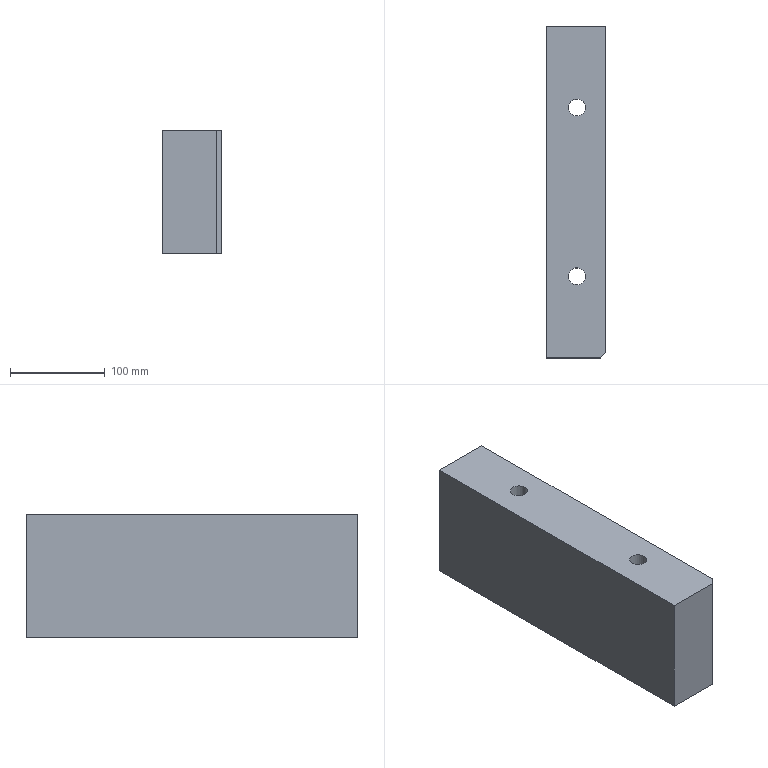Part | NX | features CC01 2 | 1 solid | 13 faces | box 63 x 350 x 130 mm | volume 2794571 mm3 | plane 7 | cylinder 4 | cone 2 | commonest cylinder face diameters 10 x2 18 x2
STEP:
#1=CARTESIAN_POINT('',(-137.5,142.,-240.5));
#2=VERTEX_POINT('',#1);
#3=CARTESIAN_POINT('',(-142.5,142.,-240.5));
#4=DIRECTION('',(0.,0.,1.));
#5=DIRECTION('',(1.,0.,0.));
#6=AXIS2_PLACEMENT_3D('',#3,#4,#5);
#7=CIRCLE('',#6,5.);
#8=EDGE_CURVE('',#2,#2,#7,.T.);
#9=ORIENTED_EDGE('',*,*,#8,.T.);
#10=EDGE_LOOP('',(#9));
#11=FACE_BOUND('',#10,.T.);
#12=CARTESIAN_POINT('',(-133.5,89.,-240.5));
#13=VERTEX_POINT('',#12);
#14=CARTESIAN_POINT('',(-142.5,89.,-240.5));
#15=DIRECTION('',(0.,0.,1.));
#16=DIRECTION('',(1.,0.,0.));
#17=AXIS2_PLACEMENT_3D('',#14,#15,#16);
#18=CIRCLE('',#17,9.);
#19=EDGE_CURVE('',#13,#13,#18,.T.);
#20=ORIENTED_EDGE('',*,*,#19,.T.);
#21=EDGE_LOOP('',(#20));
#22=FACE_BOUND('',#21,.T.);
#23=CARTESIAN_POINT('',(-112.,-169.,-240.5));
#24=VERTEX_POINT('',#23);
#25=CARTESIAN_POINT('',(-112.,175.,-240.5));
#26=VERTEX_POINT('',#25);
#27=CARTESIAN_POINT('',(-112.,0.,-240.5));
#28=DIRECTION('',(0.,1.,0.));
#29=VECTOR('',#28,1000.);
#30=LINE('',#27,#29);
#31=EDGE_CURVE('',#24,#26,#30,.T.);
#32=ORIENTED_EDGE('',*,*,#31,.F.);
#33=CARTESIAN_POINT('',(-118.,-175.,-240.5));
#34=VERTEX_POINT('',#33);
#35=CARTESIAN_POINT('',(-43.25,-100.25,-240.5));
#36=DIRECTION('',(0.7071,0.7071,0.));
#37=VECTOR('',#36,1000.);
#38=LINE('',#35,#37);
#39=EDGE_CURVE('',#24,#34,#38,.F.);
#40=ORIENTED_EDGE('',*,*,#39,.T.);
#41=CARTESIAN_POINT('',(-175.,-175.,-240.5));
#42=VERTEX_POINT('',#41);
#43=CARTESIAN_POINT('',(-143.5,-175.,-240.5));
#44=DIRECTION('',(1.,0.,0.));
#45=VECTOR('',#44,1000.);
#46=LINE('',#43,#45);
#47=EDGE_CURVE('',#42,#34,#46,.T.);
#48=ORIENTED_EDGE('',*,*,#47,.F.);
#49=CARTESIAN_POINT('',(-175.,175.,-240.5));
#50=VERTEX_POINT('',#49);
#51=CARTESIAN_POINT('',(-175.,0.,-240.5));
#52=DIRECTION('',(0.,-1.,0.));
#53=VECTOR('',#52,1000.);
#54=LINE('',#51,#53);
#55=EDGE_CURVE('',#50,#42,#54,.T.);
#56=ORIENTED_EDGE('',*,*,#55,.F.);
#57=CARTESIAN_POINT('',(-143.5,175.,-240.5));
#58=DIRECTION('',(-1.,0.,0.));
#59=VECTOR('',#58,1000.);
#60=LINE('',#57,#59);
#61=EDGE_CURVE('',#26,#50,#60,.T.);
#62=ORIENTED_EDGE('',*,*,#61,.F.);
#63=EDGE_LOOP('',(#32,#40,#48,#56,#62));
#64=FACE_BOUND('',#63,.T.);
#65=CARTESIAN_POINT('',(-133.5,-89.,-240.5));
#66=VERTEX_POINT('',#65);
#67=CARTESIAN_POINT('',(-142.5,-89.,-240.5));
#68=DIRECTION('',(0.,0.,1.));
#69=DIRECTION('',(1.,0.,0.));
#70=AXIS2_PLACEMENT_3D('',#67,#68,#69);
#71=CIRCLE('',#70,9.);
#72=EDGE_CURVE('',#66,#66,#71,.T.);
#73=ORIENTED_EDGE('',*,*,#72,.T.);
#74=EDGE_LOOP('',(#73));
#75=FACE_BOUND('',#74,.T.);
#76=CARTESIAN_POINT('',(-137.5,-142.,-240.5));
#77=VERTEX_POINT('',#76);
#78=CARTESIAN_POINT('',(-142.5,-142.,-240.5));
#79=DIRECTION('',(0.,0.,1.));
#80=DIRECTION('',(1.,0.,0.));
#81=AXIS2_PLACEMENT_3D('',#78,#79,#80);
#82=CIRCLE('',#81,5.);
#83=EDGE_CURVE('',#77,#77,#82,.T.);
#84=ORIENTED_EDGE('',*,*,#83,.T.);
#85=EDGE_LOOP('',(#84));
#86=FACE_BOUND('',#85,.T.);
#87=CARTESIAN_POINT('',(-143.5,0.,-240.5));
#88=DIRECTION('',(0.,0.,-1.));
#89=DIRECTION('',(-1.,0.,0.));
#90=AXIS2_PLACEMENT_3D('',#87,#88,#89);
#91=PLANE('',#90);
#92=ADVANCED_FACE('',(#11,#22,#64,#75,#86),#91,.T.);
#93=CARTESIAN_POINT('',(-133.5,89.,-110.5));
#94=VERTEX_POINT('',#93);
#95=CARTESIAN_POINT('',(-142.5,89.,-110.5));
#96=DIRECTION('',(0.,0.,-1.));
#97=DIRECTION('',(1.,0.,0.));
#98=AXIS2_PLACEMENT_3D('',#95,#96,#97);
#99=CIRCLE('',#98,9.);
#100=EDGE_CURVE('',#94,#94,#99,.T.);
#101=ORIENTED_EDGE('',*,*,#100,.T.);
#102=EDGE_LOOP('',(#101));
#103=FACE_BOUND('',#102,.T.);
#104=CARTESIAN_POINT('',(-118.,-175.,-110.5));
#105=VERTEX_POINT('',#104);
#106=CARTESIAN_POINT('',(-175.,-175.,-110.5));
#107=VERTEX_POINT('',#106);
#108=CARTESIAN_POINT('',(-143.5,-175.,-110.5));
#109=DIRECTION('',(-1.,0.,0.));
#110=VECTOR('',#109,1000.);
#111=LINE('',#108,#110);
#112=EDGE_CURVE('',#105,#107,#111,.T.);
#113=ORIENTED_EDGE('',*,*,#112,.F.);
#114=CARTESIAN_POINT('',(-112.,-169.,-110.5));
#115=VERTEX_POINT('',#114);
#116=CARTESIAN_POINT('',(-43.25,-100.25,-110.5));
#117=DIRECTION('',(-0.7071,-0.7071,0.));
#118=VECTOR('',#117,1000.);
#119=LINE('',#116,#118);
#120=EDGE_CURVE('',#105,#115,#119,.F.);
#121=ORIENTED_EDGE('',*,*,#120,.T.);
#122=CARTESIAN_POINT('',(-112.,175.,-110.5));
#123=VERTEX_POINT('',#122);
#124=CARTESIAN_POINT('',(-112.,0.,-110.5));
#125=DIRECTION('',(0.,-1.,0.));
#126=VECTOR('',#125,1000.);
#127=LINE('',#124,#126);
#128=EDGE_CURVE('',#123,#115,#127,.T.);
#129=ORIENTED_EDGE('',*,*,#128,.F.);
#130=CARTESIAN_POINT('',(-175.,175.,-110.5));
#131=VERTEX_POINT('',#130);
#132=CARTESIAN_POINT('',(-143.5,175.,-110.5));
#133=DIRECTION('',(1.,0.,0.));
#134=VECTOR('',#133,1000.);
#135=LINE('',#132,#134);
#136=EDGE_CURVE('',#131,#123,#135,.T.);
#137=ORIENTED_EDGE('',*,*,#136,.F.);
#138=CARTESIAN_POINT('',(-175.,0.,-110.5));
#139=DIRECTION('',(0.,1.,0.));
#140=VECTOR('',#139,1000.);
#141=LINE('',#138,#140);
#142=EDGE_CURVE('',#107,#131,#141,.T.);
#143=ORIENTED_EDGE('',*,*,#142,.F.);
#144=EDGE_LOOP('',(#113,#121,#129,#137,#143));
#145=FACE_BOUND('',#144,.T.);
#146=CARTESIAN_POINT('',(-133.5,-89.,-110.5));
#147=VERTEX_POINT('',#146);
#148=CARTESIAN_POINT('',(-142.5,-89.,-110.5));
#149=DIRECTION('',(0.,0.,-1.));
#150=DIRECTION('',(1.,0.,0.));
#151=AXIS2_PLACEMENT_3D('',#148,#149,#150);
#152=CIRCLE('',#151,9.);
#153=EDGE_CURVE('',#147,#147,#152,.T.);
#154=ORIENTED_EDGE('',*,*,#153,.T.);
#155=EDGE_LOOP('',(#154));
#156=FACE_BOUND('',#155,.T.);
#157=CARTESIAN_POINT('',(-143.5,0.,-110.5));
#158=DIRECTION('',(0.,0.,1.));
#159=DIRECTION('',(1.,0.,0.));
#160=AXIS2_PLACEMENT_3D('',#157,#158,#159);
#161=PLANE('',#160);
#162=ADVANCED_FACE('',(#103,#145,#156),#161,.T.);
#163=ORIENTED_EDGE('',*,*,#47,.T.);
#164=CARTESIAN_POINT('',(-118.,-175.,-240.5));
#165=DIRECTION('',(0.,0.,1.));
#166=VECTOR('',#165,1000.);
#167=LINE('',#164,#166);
#168=EDGE_CURVE('',#34,#105,#167,.T.);
#169=ORIENTED_EDGE('',*,*,#168,.T.);
#170=ORIENTED_EDGE('',*,*,#112,.T.);
#171=CARTESIAN_POINT('',(-175.,-175.,-240.5));
#172=DIRECTION('',(0.,0.,1.));
#173=VECTOR('',#172,1000.);
#174=LINE('',#171,#173);
#175=EDGE_CURVE('',#42,#107,#174,.T.);
#176=ORIENTED_EDGE('',*,*,#175,.F.);
#177=EDGE_LOOP('',(#163,#169,#170,#176));
#178=FACE_BOUND('',#177,.T.);
#179=CARTESIAN_POINT('',(-143.5,-175.,-240.5));
#180=DIRECTION('',(0.,-1.,0.));
#181=DIRECTION('',(0.,0.,-1.));
#182=AXIS2_PLACEMENT_3D('',#179,#180,#181);
#183=PLANE('',#182);
#184=ADVANCED_FACE('',(#178),#183,.T.);
#185=ORIENTED_EDGE('',*,*,#175,.T.);
#186=ORIENTED_EDGE('',*,*,#142,.T.);
#187=CARTESIAN_POINT('',(-175.,175.,-240.5));
#188=DIRECTION('',(0.,0.,1.));
#189=VECTOR('',#188,1000.);
#190=LINE('',#187,#189);
#191=EDGE_CURVE('',#50,#131,#190,.T.);
#192=ORIENTED_EDGE('',*,*,#191,.F.);
#193=ORIENTED_EDGE('',*,*,#55,.T.);
#194=EDGE_LOOP('',(#185,#186,#192,#193));
#195=FACE_BOUND('',#194,.T.);
#196=CARTESIAN_POINT('',(-175.,0.,-240.5));
#197=DIRECTION('',(-1.,0.,0.));
#198=DIRECTION('',(0.,0.,1.));
#199=AXIS2_PLACEMENT_3D('',#196,#197,#198);
#200=PLANE('',#199);
#201=ADVANCED_FACE('',(#195),#200,.T.);
#202=ORIENTED_EDGE('',*,*,#191,.T.);
#203=ORIENTED_EDGE('',*,*,#136,.T.);
#204=CARTESIAN_POINT('',(-112.,175.,-240.5));
#205=DIRECTION('',(0.,0.,1.));
#206=VECTOR('',#205,1000.);
#207=LINE('',#204,#206);
#208=EDGE_CURVE('',#26,#123,#207,.T.);
#209=ORIENTED_EDGE('',*,*,#208,.F.);
#210=ORIENTED_EDGE('',*,*,#61,.T.);
#211=EDGE_LOOP('',(#202,#203,#209,#210));
#212=FACE_BOUND('',#211,.T.);
#213=CARTESIAN_POINT('',(-143.5,175.,-240.5));
#214=DIRECTION('',(0.,1.,0.));
#215=DIRECTION('',(0.,0.,1.));
#216=AXIS2_PLACEMENT_3D('',#213,#214,#215);
#217=PLANE('',#216);
#218=ADVANCED_FACE('',(#212),#217,.T.);
#219=ORIENTED_EDGE('',*,*,#128,.T.);
#220=CARTESIAN_POINT('',(-112.,-169.,-240.5));
#221=DIRECTION('',(0.,0.,-1.));
#222=VECTOR('',#221,1000.);
#223=LINE('',#220,#222);
#224=EDGE_CURVE('',#115,#24,#223,.T.);
#225=ORIENTED_EDGE('',*,*,#224,.T.);
#226=ORIENTED_EDGE('',*,*,#31,.T.);
#227=ORIENTED_EDGE('',*,*,#208,.T.);
#228=EDGE_LOOP('',(#219,#225,#226,#227));
#229=FACE_BOUND('',#228,.T.);
#230=CARTESIAN_POINT('',(-112.,0.,-240.5));
#231=DIRECTION('',(1.,0.,0.));
#232=DIRECTION('',(0.,0.,-1.));
#233=AXIS2_PLACEMENT_3D('',#230,#231,#232);
#234=PLANE('',#233);
#235=ADVANCED_FACE('',(#229),#234,.T.);
#236=ORIENTED_EDGE('',*,*,#100,.F.);
#237=EDGE_LOOP('',(#236));
#238=FACE_BOUND('',#237,.T.);
#239=ORIENTED_EDGE('',*,*,#19,.F.);
#240=EDGE_LOOP('',(#239));
#241=FACE_BOUND('',#240,.T.);
#242=CARTESIAN_POINT('',(-142.5,89.,-240.5));
#243=DIRECTION('',(0.,0.,1.));
#244=DIRECTION('',(1.,0.,0.));
#245=AXIS2_PLACEMENT_3D('',#242,#243,#244);
#246=CYLINDRICAL_SURFACE('',#245,9.);
#247=ADVANCED_FACE('',(#238,#241),#246,.F.);
#248=ORIENTED_EDGE('',*,*,#153,.F.);
#249=EDGE_LOOP('',(#248));
#250=FACE_BOUND('',#249,.T.);
#251=ORIENTED_EDGE('',*,*,#72,.F.);
#252=EDGE_LOOP('',(#251));
#253=FACE_BOUND('',#252,.T.);
#254=CARTESIAN_POINT('',(-142.5,-89.,-240.5));
#255=DIRECTION('',(0.,0.,1.));
#256=DIRECTION('',(1.,0.,0.));
#257=AXIS2_PLACEMENT_3D('',#254,#255,#256);
#258=CYLINDRICAL_SURFACE('',#257,9.);
#259=ADVANCED_FACE('',(#250,#253),#258,.F.);
#260=CARTESIAN_POINT('',(-137.5,142.,-219.5));
#261=VERTEX_POINT('',#260);
#262=CARTESIAN_POINT('',(-142.5,142.,-219.5));
#263=DIRECTION('',(0.,0.,1.));
#264=DIRECTION('',(1.,0.,0.));
#265=AXIS2_PLACEMENT_3D('',#262,#263,#264);
#266=CIRCLE('',#265,5.);
#267=EDGE_CURVE('',#261,#261,#266,.T.);
#268=ORIENTED_EDGE('',*,*,#267,.T.);
#269=EDGE_LOOP('',(#268));
#270=FACE_BOUND('',#269,.T.);
#271=ORIENTED_EDGE('',*,*,#8,.F.);
#272=EDGE_LOOP('',(#271));
#273=FACE_BOUND('',#272,.T.);
#274=CARTESIAN_POINT('',(-142.5,142.,-240.5));
#275=DIRECTION('',(0.,0.,1.));
#276=DIRECTION('',(1.,0.,0.));
#277=AXIS2_PLACEMENT_3D('',#274,#275,#276);
#278=CYLINDRICAL_SURFACE('',#277,5.);
#279=ADVANCED_FACE('',(#270,#273),#278,.F.);
#280=CARTESIAN_POINT('',(-137.5,-142.,-219.5));
#281=VERTEX_POINT('',#280);
#282=CARTESIAN_POINT('',(-142.5,-142.,-219.5));
#283=DIRECTION('',(0.,0.,1.));
#284=DIRECTION('',(1.,0.,0.));
#285=AXIS2_PLACEMENT_3D('',#282,#283,#284);
#286=CIRCLE('',#285,5.);
#287=EDGE_CURVE('',#281,#281,#286,.T.);
#288=ORIENTED_EDGE('',*,*,#287,.T.);
#289=EDGE_LOOP('',(#288));
#290=FACE_BOUND('',#289,.T.);
#291=ORIENTED_EDGE('',*,*,#83,.F.);
#292=EDGE_LOOP('',(#291));
#293=FACE_BOUND('',#292,.T.);
#294=CARTESIAN_POINT('',(-142.5,-142.,-240.5));
#295=DIRECTION('',(0.,0.,1.));
#296=DIRECTION('',(1.,0.,0.));
#297=AXIS2_PLACEMENT_3D('',#294,#295,#296);
#298=CYLINDRICAL_SURFACE('',#297,5.);
#299=ADVANCED_FACE('',(#290,#293),#298,.F.);
#300=ORIENTED_EDGE('',*,*,#267,.F.);
#301=EDGE_LOOP('',(#300));
#302=FACE_BOUND('',#301,.T.);
#303=CARTESIAN_POINT('',(-142.5,142.,-217.05));
#304=VERTEX_POINT('',#303);
#305=VERTEX_LOOP('',#304);
#306=FACE_BOUND('',#305,.T.);
#307=CARTESIAN_POINT('',(-142.5,142.,-217.05));
#308=DIRECTION('',(0.,0.,-1.));
#309=DIRECTION('',(1.,0.,0.));
#310=AXIS2_PLACEMENT_3D('',#307,#308,#309);
#311=CONICAL_SURFACE('',#310,0.,1.115);
#312=ADVANCED_FACE('',(#302,#306),#311,.F.);
#313=ORIENTED_EDGE('',*,*,#287,.F.);
#314=EDGE_LOOP('',(#313));
#315=FACE_BOUND('',#314,.T.);
#316=CARTESIAN_POINT('',(-142.5,-142.,-217.05));
#317=VERTEX_POINT('',#316);
#318=VERTEX_LOOP('',#317);
#319=FACE_BOUND('',#318,.T.);
#320=CARTESIAN_POINT('',(-142.5,-142.,-217.05));
#321=DIRECTION('',(0.,0.,-1.));
#322=DIRECTION('',(1.,0.,0.));
#323=AXIS2_PLACEMENT_3D('',#320,#321,#322);
#324=CONICAL_SURFACE('',#323,0.,1.115);
#325=ADVANCED_FACE('',(#315,#319),#324,.F.);
#326=ORIENTED_EDGE('',*,*,#39,.F.);
#327=ORIENTED_EDGE('',*,*,#224,.F.);
#328=ORIENTED_EDGE('',*,*,#120,.F.);
#329=ORIENTED_EDGE('',*,*,#168,.F.);
#330=EDGE_LOOP('',(#326,#327,#328,#329));
#331=FACE_BOUND('',#330,.T.);
#332=CARTESIAN_POINT('',(-118.,-175.,-240.5));
#333=DIRECTION('',(-0.7071,0.7071,0.));
#334=DIRECTION('',(0.,0.,1.));
#335=AXIS2_PLACEMENT_3D('',#332,#333,#334);
#336=PLANE('',#335);
#337=ADVANCED_FACE('',(#331),#336,.F.);
#338=CLOSED_SHELL('',(#92,#162,#184,#201,#218,#235,#247,#259,#279,#299,#312,#325,#337));
#339=MANIFOLD_SOLID_BREP('',#338);
#340=(LENGTH_UNIT()NAMED_UNIT(*)SI_UNIT(.MILLI.,.METRE.));
#341=UNCERTAINTY_MEASURE_WITH_UNIT(LENGTH_MEASURE(0.00001),#340,'','');
#342=(NAMED_UNIT(*)PLANE_ANGLE_UNIT()SI_UNIT($,.RADIAN.));
#343=(NAMED_UNIT(*)SI_UNIT($,.STERADIAN.)SOLID_ANGLE_UNIT());
#344=(GEOMETRIC_REPRESENTATION_CONTEXT(3)GLOBAL_UNCERTAINTY_ASSIGNED_CONTEXT((#341))GLOBAL_UNIT_ASSIGNED_CONTEXT((#340,#342,#343))REPRESENTATION_CONTEXT('',''));
#345=ADVANCED_BREP_SHAPE_REPRESENTATION('',(#339),#344);